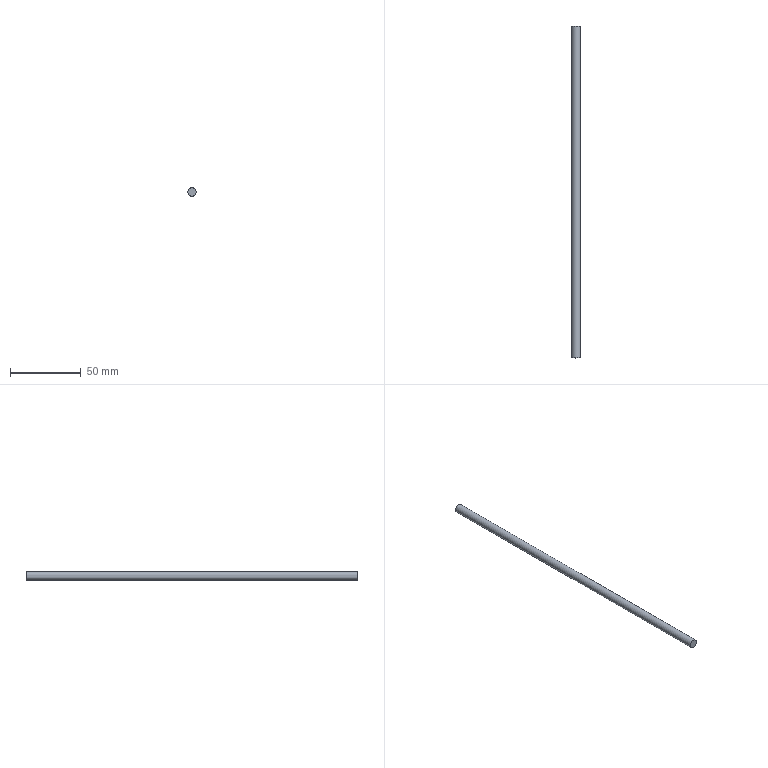Part | NX | features solid 2 | 1 solid | 3 faces | box 6 x 234 x 6 mm | volume 6616 mm3 | plane 2 | cylinder 1 | commonest cylinder face diameters 6 x1
STEP:
#1=CARTESIAN_POINT('',(0.,59.,-84.));
#2=VERTEX_POINT('',#1);
#3=CARTESIAN_POINT('',(0.,59.,-87.));
#4=DIRECTION('',(0.,1.,0.));
#5=DIRECTION('',(0.,0.,1.));
#6=AXIS2_PLACEMENT_3D('',#3,#4,#5);
#7=CIRCLE('',#6,3.);
#8=EDGE_CURVE('',#2,#2,#7,.F.);
#9=ORIENTED_EDGE('',*,*,#8,.F.);
#10=EDGE_LOOP('',(#9));
#11=FACE_BOUND('',#10,.T.);
#12=CARTESIAN_POINT('',(0.,59.,-87.));
#13=DIRECTION('',(0.,1.,0.));
#14=DIRECTION('',(0.,0.,1.));
#15=AXIS2_PLACEMENT_3D('',#12,#13,#14);
#16=PLANE('',#15);
#17=ADVANCED_FACE('',(#11),#16,.T.);
#18=CARTESIAN_POINT('',(0.,-175.,-90.));
#19=VERTEX_POINT('',#18);
#20=CARTESIAN_POINT('',(0.,-175.,-87.));
#21=DIRECTION('',(0.,-1.,0.));
#22=DIRECTION('',(0.,0.,-1.));
#23=AXIS2_PLACEMENT_3D('',#20,#21,#22);
#24=CIRCLE('',#23,3.);
#25=EDGE_CURVE('',#19,#19,#24,.F.);
#26=ORIENTED_EDGE('',*,*,#25,.F.);
#27=EDGE_LOOP('',(#26));
#28=FACE_BOUND('',#27,.T.);
#29=CARTESIAN_POINT('',(0.,-175.,-110.5));
#30=DIRECTION('',(0.,-1.,0.));
#31=DIRECTION('',(0.,0.,-1.));
#32=AXIS2_PLACEMENT_3D('',#29,#30,#31);
#33=PLANE('',#32);
#34=ADVANCED_FACE('',(#28),#33,.T.);
#35=ORIENTED_EDGE('',*,*,#8,.T.);
#36=EDGE_LOOP('',(#35));
#37=FACE_BOUND('',#36,.T.);
#38=ORIENTED_EDGE('',*,*,#25,.T.);
#39=EDGE_LOOP('',(#38));
#40=FACE_BOUND('',#39,.T.);
#41=CARTESIAN_POINT('',(0.,0.,-87.));
#42=DIRECTION('',(0.,1.,0.));
#43=DIRECTION('',(1.,0.,0.));
#44=AXIS2_PLACEMENT_3D('',#41,#42,#43);
#45=CYLINDRICAL_SURFACE('',#44,3.);
#46=ADVANCED_FACE('',(#37,#40),#45,.T.);
#47=CLOSED_SHELL('',(#17,#34,#46));
#48=MANIFOLD_SOLID_BREP('',#47);
#49=(LENGTH_UNIT()NAMED_UNIT(*)SI_UNIT(.MILLI.,.METRE.));
#50=UNCERTAINTY_MEASURE_WITH_UNIT(LENGTH_MEASURE(0.00001),#49,'','');
#51=(NAMED_UNIT(*)PLANE_ANGLE_UNIT()SI_UNIT($,.RADIAN.));
#52=(NAMED_UNIT(*)SI_UNIT($,.STERADIAN.)SOLID_ANGLE_UNIT());
#53=(GEOMETRIC_REPRESENTATION_CONTEXT(3)GLOBAL_UNCERTAINTY_ASSIGNED_CONTEXT((#50))GLOBAL_UNIT_ASSIGNED_CONTEXT((#49,#51,#52))REPRESENTATION_CONTEXT('',''));
#54=ADVANCED_BREP_SHAPE_REPRESENTATION('',(#48),#53);